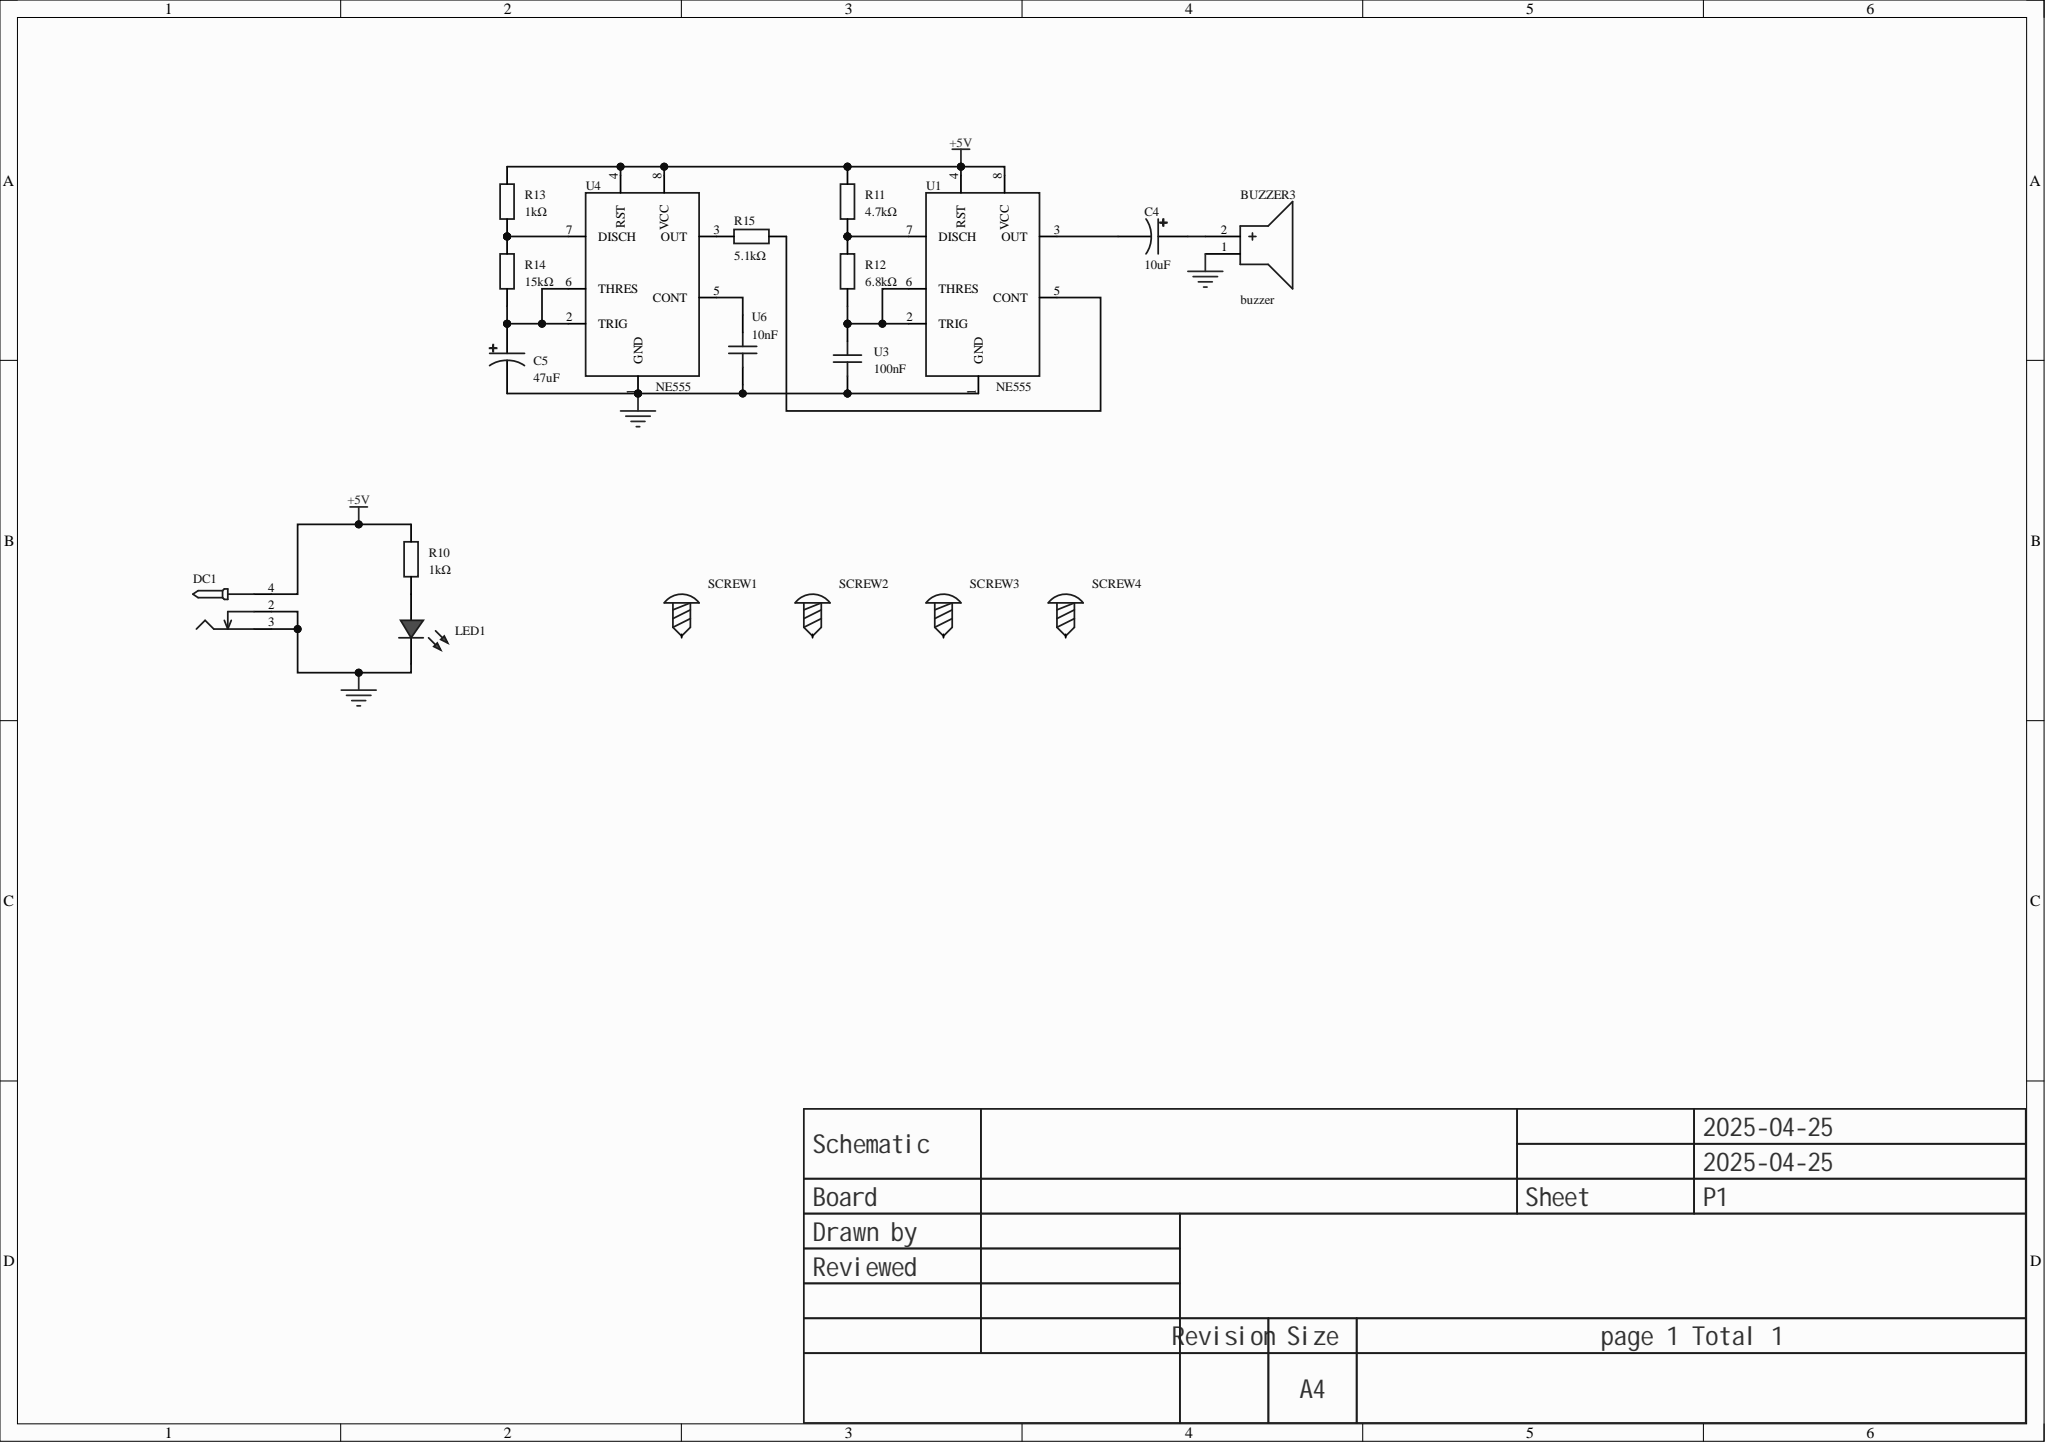Circuit board | Altium Designer | 19 parts | 12 nets
Bill of materials:
Comment,Description,Designator,Footprint,LibRef,Quantity
"buzzer","","BUZZER3","BUZ-TH_BD12.0-P6.00-D0.9-RD","buzzer","1"
"10uF","Capacitance: 4.7uF; Tolerance: ±20%; Rated voltage: 100V;","C4","CAP-TH_BD5.0-P2.00-D0.8-FD","KM475M100D11RR0VH2FP0","1"
"47uF","Capacitance: 4.7uF; Tolerance: ±20%; Rated voltage: 100V;","C5","CAP-TH_BD5.0-P2.00-D0.8-FD","KM475M100D11RR0VH2FP0","1"
"","","DC1","DC-2.0","DC-005_2.0","1"
"","","LED1","LED_TH-3mm","LED_TH-R_3mm","1"
"1kΩ","","R10, R13","Res_1/8W","Res_AXIAL-1/8W","2"
"4.7kΩ","","R11","Res_1/8W","Res_AXIAL-1/8W","1"
"6.8kΩ","","R12","Res_1/8W","Res_AXIAL-1/8W","1"
"15kΩ","","R14","Res_1/8W","Res_AXIAL-1/8W","1"
"5.1kΩ","","R15","Res_1/8W","Res_AXIAL-1/8W","1"
"","","SCREW1, SCREW2, SCREW3, SCREW4","M3螺丝","M3螺丝","4"
"NE555","NE555 single timer","U1, U4","PDIP-8_L9.6-W6.4-P2.54-LS7.9-BL-1","NE555PE4","2"
"100nF","Capacitance: 10nF; Tolerance: ±10%; Rated voltage: 50V; Temperature coefficient: X7R;","U3","CAP-TH_L4.0-W2.5-P2.50-D0.5","FK18X7R1H103K","1"
"10nF","Capacitance: 10nF; Tolerance: ±10%; Rated voltage: 50V; Temperature coefficient: X7R;","U6","CAP-TH_L4.0-W2.5-P2.50-D0.5","FK18X7R1H103K","1"
Netlist (Protel format):
[
BUZZER3
BUZ-TH_BD12.0-P6.00-D0.9-RD
buzzer



]
[
C4
CAP-TH_BD5.0-P2.00-D0.8-FD
10uF



]
[
C5
CAP-TH_BD5.0-P2.00-D0.8-FD
47uF



]
[
DC1
DC-2.0




]
[
LED1
LED_TH-3mm




]
[
R10
Res_1/8W
1kΩ



]
[
R11
Res_1/8W
4.7kΩ



]
[
R12
Res_1/8W
6.8kΩ



]
[
R13
Res_1/8W
1kΩ



]
[
R14
Res_1/8W
15kΩ



]
[
R15
Res_1/8W
5.1kΩ



]
[
SCREW1
M3螺丝




]
[
SCREW2
M3螺丝




]
[
SCREW3
M3螺丝




]
[
SCREW4
M3螺丝




]
[
U1
PDIP-8_L9.6-W6.4-P2.54-LS7.9-BL-1
NE555



]
[
U3
CAP-TH_L4.0-W2.5-P2.50-D0.5
100nF



]
[
U4
PDIP-8_L9.6-W6.4-P2.54-LS7.9-BL-1
NE555



]
[
U6
CAP-TH_L4.0-W2.5-P2.50-D0.5
10nF



]
(
NetU4_5
U4-5
U6-2
)
(
NetR15_2
R15-2
U4-3
)
(
NetR15_1
R15-1
U1-5
)
(
NetR13_1
R13-1
R14-2
U4-7
)
(
NetR12_1
R12-1
U1-2
U1-6
U3-2
)
(
NetR11_1
R11-1
R12-2
U1-7
)
(
NetLED1_1
LED1-1
R10-1
)
(
NetC5_1
C5-1
R14-1
U4-2
U4-6
)
(
NetC4_2
C4-2
U1-3
)
(
NetBUZZER3_2
BUZZER3-2
C4-1
)
(
GND
BUZZER3-1
C5-2
DC1-2
DC1-3
LED1-2
U1-1
U3-1
U4-1
U6-1
)
(
+5V
DC1-4
R10-2
R11-2
R13-2
U1-4
U1-8
U4-4
U4-8
)